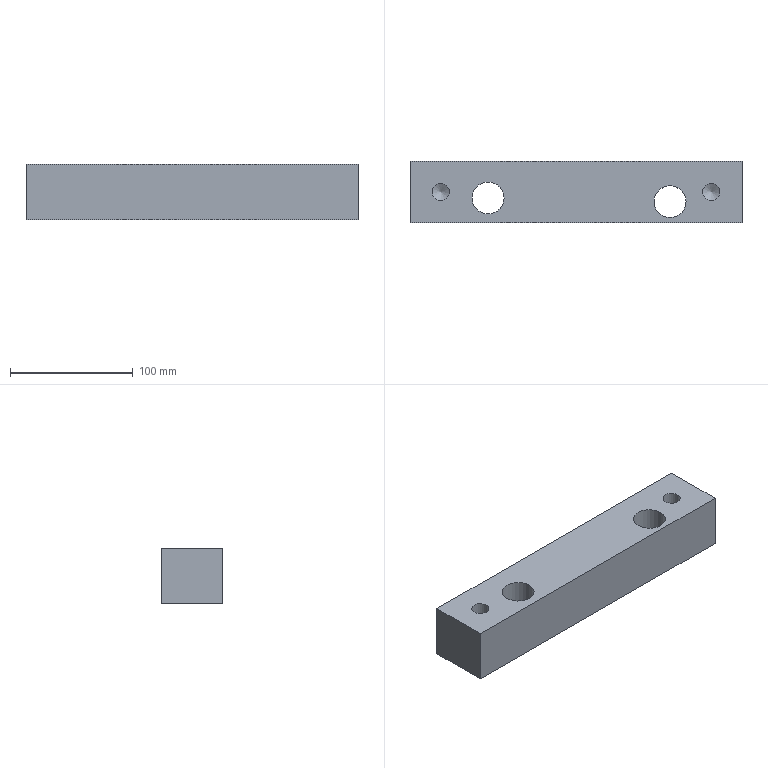Part | STEP file | 017_id2174_x_t | 1 solid | 12 faces | box 270 x 50 x 45 mm | volume 553311 mm3 | plane 6 | cylinder 4 | cone 2 | commonest cylinder face diameters 14 x2 26 x2
STEP:
#1=CARTESIAN_POINT('',(0.,0.,0.));
#2=DIRECTION('',(0.,0.,1.));
#3=DIRECTION('',(1.,0.,0.));
#4=AXIS2_PLACEMENT_3D('',#1,#2,#3);
#5=CARTESIAN_POINT('',(92.98,-48.947,230.));
#6=VERTEX_POINT('',#5);
#7=CARTESIAN_POINT('',(79.98,-48.947,230.));
#8=DIRECTION('',(0.,0.,1.));
#9=DIRECTION('',(1.,0.,0.));
#10=AXIS2_PLACEMENT_3D('',#7,#8,#9);
#11=CIRCLE('',#10,13.);
#12=CARTESIAN_POINT('',(303.5,139.,230.));
#13=DIRECTION('',(0.,0.,1.));
#14=DIRECTION('',(0.,1.,0.));
#15=AXIS2_PLACEMENT_3D('',#12,#13,#14);
#16=PLANE('',#15);
#17=CARTESIAN_POINT('',(-187.947,223.52));
#18=DIRECTION('',(0.,-1.));
#19=AXIS2_PLACEMENT_2D('',#17,#18);
#20=CIRCLE('',#19,13.);
#21=(GEOMETRIC_REPRESENTATION_CONTEXT(2)PARAMETRIC_REPRESENTATION_CONTEXT()REPRESENTATION_CONTEXT('',''));
#22=DEFINITIONAL_REPRESENTATION('',(#20),#21);
#23=PCURVE('',#16,#22);
#24=CARTESIAN_POINT('',(79.98,-48.947,360.));
#25=DIRECTION('',(0.,0.,-1.));
#26=DIRECTION('',(-1.,0.,0.));
#27=AXIS2_PLACEMENT_3D('',#24,#25,#26);
#28=CYLINDRICAL_SURFACE('',#27,13.);
#29=CARTESIAN_POINT('',(9.425,130.));
#30=DIRECTION('',(-1.,0.));
#31=VECTOR('',#30,1.);
#32=LINE('',#29,#31);
#33=(GEOMETRIC_REPRESENTATION_CONTEXT(2)PARAMETRIC_REPRESENTATION_CONTEXT()REPRESENTATION_CONTEXT('',''));
#34=DEFINITIONAL_REPRESENTATION('',(#32),#33);
#35=PCURVE('',#28,#34);
#36=SURFACE_CURVE('',#11,(#23,#35),.PCURVE_S1.);
#37=EDGE_CURVE('',#6,#6,#36,.T.);
#38=ORIENTED_EDGE('',*,*,#37,.F.);
#39=EDGE_LOOP('',(#38));
#40=FACE_BOUND('',#39,.T.);
#41=CARTESIAN_POINT('',(-55.02,-45.947,230.));
#42=VERTEX_POINT('',#41);
#43=CARTESIAN_POINT('',(-68.02,-45.947,230.));
#44=DIRECTION('',(0.,0.,1.));
#45=DIRECTION('',(1.,0.,0.));
#46=AXIS2_PLACEMENT_3D('',#43,#44,#45);
#47=CIRCLE('',#46,13.);
#48=CARTESIAN_POINT('',(-184.947,371.52));
#49=DIRECTION('',(0.,-1.));
#50=AXIS2_PLACEMENT_2D('',#48,#49);
#51=CIRCLE('',#50,13.);
#52=(GEOMETRIC_REPRESENTATION_CONTEXT(2)PARAMETRIC_REPRESENTATION_CONTEXT()REPRESENTATION_CONTEXT('',''));
#53=DEFINITIONAL_REPRESENTATION('',(#51),#52);
#54=PCURVE('',#16,#53);
#55=CARTESIAN_POINT('',(-68.02,-45.947,360.));
#56=DIRECTION('',(0.,0.,-1.));
#57=DIRECTION('',(-1.,0.,0.));
#58=AXIS2_PLACEMENT_3D('',#55,#56,#57);
#59=CYLINDRICAL_SURFACE('',#58,13.);
#60=CARTESIAN_POINT('',(9.425,130.));
#61=DIRECTION('',(-1.,0.));
#62=VECTOR('',#61,1.);
#63=LINE('',#60,#62);
#64=(GEOMETRIC_REPRESENTATION_CONTEXT(2)PARAMETRIC_REPRESENTATION_CONTEXT()REPRESENTATION_CONTEXT('',''));
#65=DEFINITIONAL_REPRESENTATION('',(#63),#64);
#66=PCURVE('',#59,#65);
#67=SURFACE_CURVE('',#47,(#54,#66),.PCURVE_S1.);
#68=EDGE_CURVE('',#42,#42,#67,.T.);
#69=ORIENTED_EDGE('',*,*,#68,.F.);
#70=EDGE_LOOP('',(#69));
#71=FACE_BOUND('',#70,.T.);
#72=CARTESIAN_POINT('',(-106.5,-48.,230.));
#73=VERTEX_POINT('',#72);
#74=CARTESIAN_POINT('',(-106.5,-34.,230.));
#75=VERTEX_POINT('',#74);
#76=CARTESIAN_POINT('',(-106.5,-41.,230.));
#77=DIRECTION('',(0.,0.,1.));
#78=DIRECTION('',(0.,-1.,0.));
#79=AXIS2_PLACEMENT_3D('',#76,#77,#78);
#80=CIRCLE('',#79,7.);
#81=CARTESIAN_POINT('',(-180.,410.));
#82=DIRECTION('',(-1.,0.));
#83=AXIS2_PLACEMENT_2D('',#81,#82);
#84=CIRCLE('',#83,7.);
#85=(GEOMETRIC_REPRESENTATION_CONTEXT(2)PARAMETRIC_REPRESENTATION_CONTEXT()REPRESENTATION_CONTEXT('',''));
#86=DEFINITIONAL_REPRESENTATION('',(#84),#85);
#87=PCURVE('',#16,#86);
#88=CARTESIAN_POINT('',(-106.5,-41.,279.));
#89=DIRECTION('',(0.,0.,-1.));
#90=DIRECTION('',(0.,1.,0.));
#91=AXIS2_PLACEMENT_3D('',#88,#89,#90);
#92=CYLINDRICAL_SURFACE('',#91,7.);
#93=CARTESIAN_POINT('',(3.142,49.));
#94=DIRECTION('',(-1.,0.));
#95=VECTOR('',#94,1.);
#96=LINE('',#93,#95);
#97=(GEOMETRIC_REPRESENTATION_CONTEXT(2)PARAMETRIC_REPRESENTATION_CONTEXT()REPRESENTATION_CONTEXT('',''));
#98=DEFINITIONAL_REPRESENTATION('',(#96),#97);
#99=PCURVE('',#92,#98);
#100=SURFACE_CURVE('',#80,(#87,#99),.PCURVE_S1.);
#101=EDGE_CURVE('',#73,#75,#100,.T.);
#102=ORIENTED_EDGE('',*,*,#101,.F.);
#103=CARTESIAN_POINT('',(-106.5,-41.,230.));
#104=DIRECTION('',(0.,0.,1.));
#105=DIRECTION('',(0.,-1.,0.));
#106=AXIS2_PLACEMENT_3D('',#103,#104,#105);
#107=CIRCLE('',#106,7.);
#108=CARTESIAN_POINT('',(-180.,410.));
#109=DIRECTION('',(-1.,0.));
#110=AXIS2_PLACEMENT_2D('',#108,#109);
#111=CIRCLE('',#110,7.);
#112=(GEOMETRIC_REPRESENTATION_CONTEXT(2)PARAMETRIC_REPRESENTATION_CONTEXT()REPRESENTATION_CONTEXT('',''));
#113=DEFINITIONAL_REPRESENTATION('',(#111),#112);
#114=PCURVE('',#16,#113);
#115=CARTESIAN_POINT('',(9.425,49.));
#116=DIRECTION('',(-1.,0.));
#117=VECTOR('',#116,1.);
#118=LINE('',#115,#117);
#119=(GEOMETRIC_REPRESENTATION_CONTEXT(2)PARAMETRIC_REPRESENTATION_CONTEXT()REPRESENTATION_CONTEXT('',''));
#120=DEFINITIONAL_REPRESENTATION('',(#118),#119);
#121=PCURVE('',#92,#120);
#122=SURFACE_CURVE('',#107,(#114,#121),.PCURVE_S1.);
#123=EDGE_CURVE('',#75,#73,#122,.T.);
#124=ORIENTED_EDGE('',*,*,#123,.F.);
#125=EDGE_LOOP('',(#102,#124));
#126=FACE_BOUND('',#125,.T.);
#127=CARTESIAN_POINT('',(113.5,-48.,230.));
#128=VERTEX_POINT('',#127);
#129=CARTESIAN_POINT('',(113.5,-34.,230.));
#130=VERTEX_POINT('',#129);
#131=CARTESIAN_POINT('',(113.5,-41.,230.));
#132=DIRECTION('',(0.,0.,-1.));
#133=DIRECTION('',(0.,-1.,0.));
#134=AXIS2_PLACEMENT_3D('',#131,#132,#133);
#135=CIRCLE('',#134,7.);
#136=CARTESIAN_POINT('',(-187.,190.));
#137=CARTESIAN_POINT('',(-187.,202.124));
#138=CARTESIAN_POINT('',(-176.5,196.062));
#139=CARTESIAN_POINT('',(-166.,190.));
#140=CARTESIAN_POINT('',(-176.5,183.938));
#141=CARTESIAN_POINT('',(-187.,177.876));
#142=CARTESIAN_POINT('',(-187.,190.));
#143=(BOUNDED_CURVE()B_SPLINE_CURVE(2,(#136,#137,#138,#139,#140,#141,#142),.UNSPECIFIED.,.T.,.F.)B_SPLINE_CURVE_WITH_KNOTS((1,2,2,2,2,1),(-2.094,0.,2.094,4.189,6.283,8.378),.UNSPECIFIED.)CURVE()GEOMETRIC_REPRESENTATION_ITEM()RATIONAL_B_SPLINE_CURVE((1.,0.5,1.,0.5,1.,0.5,1.))REPRESENTATION_ITEM(''));
#144=(GEOMETRIC_REPRESENTATION_CONTEXT(2)PARAMETRIC_REPRESENTATION_CONTEXT()REPRESENTATION_CONTEXT('',''));
#145=DEFINITIONAL_REPRESENTATION('',(#143),#144);
#146=PCURVE('',#16,#145);
#147=CARTESIAN_POINT('',(113.5,-41.,279.));
#148=DIRECTION('',(0.,0.,-1.));
#149=DIRECTION('',(0.,1.,0.));
#150=AXIS2_PLACEMENT_3D('',#147,#148,#149);
#151=CYLINDRICAL_SURFACE('',#150,7.);
#152=CARTESIAN_POINT('',(3.142,49.));
#153=DIRECTION('',(1.,0.));
#154=VECTOR('',#153,1.);
#155=LINE('',#152,#154);
#156=(GEOMETRIC_REPRESENTATION_CONTEXT(2)PARAMETRIC_REPRESENTATION_CONTEXT()REPRESENTATION_CONTEXT('',''));
#157=DEFINITIONAL_REPRESENTATION('',(#155),#156);
#158=PCURVE('',#151,#157);
#159=SURFACE_CURVE('',#135,(#146,#158),.PCURVE_S1.);
#160=EDGE_CURVE('',#128,#130,#159,.T.);
#161=ORIENTED_EDGE('',*,*,#160,.T.);
#162=CARTESIAN_POINT('',(113.5,-41.,230.));
#163=DIRECTION('',(0.,0.,-1.));
#164=DIRECTION('',(0.,-1.,0.));
#165=AXIS2_PLACEMENT_3D('',#162,#163,#164);
#166=CIRCLE('',#165,7.);
#167=CARTESIAN_POINT('',(-187.,190.));
#168=CARTESIAN_POINT('',(-187.,202.124));
#169=CARTESIAN_POINT('',(-176.5,196.062));
#170=CARTESIAN_POINT('',(-166.,190.));
#171=CARTESIAN_POINT('',(-176.5,183.938));
#172=CARTESIAN_POINT('',(-187.,177.876));
#173=CARTESIAN_POINT('',(-187.,190.));
#174=(BOUNDED_CURVE()B_SPLINE_CURVE(2,(#167,#168,#169,#170,#171,#172,#173),.UNSPECIFIED.,.T.,.F.)B_SPLINE_CURVE_WITH_KNOTS((1,2,2,2,2,1),(-2.094,0.,2.094,4.189,6.283,8.378),.UNSPECIFIED.)CURVE()GEOMETRIC_REPRESENTATION_ITEM()RATIONAL_B_SPLINE_CURVE((1.,0.5,1.,0.5,1.,0.5,1.))REPRESENTATION_ITEM(''));
#175=(GEOMETRIC_REPRESENTATION_CONTEXT(2)PARAMETRIC_REPRESENTATION_CONTEXT()REPRESENTATION_CONTEXT('',''));
#176=DEFINITIONAL_REPRESENTATION('',(#174),#175);
#177=PCURVE('',#16,#176);
#178=CARTESIAN_POINT('',(-3.142,49.));
#179=DIRECTION('',(1.,0.));
#180=VECTOR('',#179,1.);
#181=LINE('',#178,#180);
#182=(GEOMETRIC_REPRESENTATION_CONTEXT(2)PARAMETRIC_REPRESENTATION_CONTEXT()REPRESENTATION_CONTEXT('',''));
#183=DEFINITIONAL_REPRESENTATION('',(#181),#182);
#184=PCURVE('',#151,#183);
#185=SURFACE_CURVE('',#166,(#177,#184),.PCURVE_S1.);
#186=EDGE_CURVE('',#130,#128,#185,.T.);
#187=ORIENTED_EDGE('',*,*,#186,.T.);
#188=EDGE_LOOP('',(#161,#187));
#189=FACE_BOUND('',#188,.T.);
#190=CARTESIAN_POINT('',(-131.5,-16.,230.));
#191=VERTEX_POINT('',#190);
#192=CARTESIAN_POINT('',(-131.5,-66.,230.));
#193=VERTEX_POINT('',#192);
#194=CARTESIAN_POINT('',(-131.5,-66.,230.));
#195=DIRECTION('',(0.,-1.,0.));
#196=VECTOR('',#195,1.);
#197=LINE('',#194,#196);
#198=CARTESIAN_POINT('',(-205.,435.));
#199=DIRECTION('',(-1.,0.));
#200=VECTOR('',#199,1.);
#201=LINE('',#198,#200);
#202=(GEOMETRIC_REPRESENTATION_CONTEXT(2)PARAMETRIC_REPRESENTATION_CONTEXT()REPRESENTATION_CONTEXT('',''));
#203=DEFINITIONAL_REPRESENTATION('',(#201),#202);
#204=PCURVE('',#16,#203);
#205=CARTESIAN_POINT('',(-131.5,-66.,428.5));
#206=DIRECTION('',(-1.,0.,0.));
#207=DIRECTION('',(0.,0.,1.));
#208=AXIS2_PLACEMENT_3D('',#205,#206,#207);
#209=PLANE('',#208);
#210=CARTESIAN_POINT('',(-198.5,0.));
#211=DIRECTION('',(0.,-1.));
#212=VECTOR('',#211,1.);
#213=LINE('',#210,#212);
#214=(GEOMETRIC_REPRESENTATION_CONTEXT(2)PARAMETRIC_REPRESENTATION_CONTEXT()REPRESENTATION_CONTEXT('',''));
#215=DEFINITIONAL_REPRESENTATION('',(#213),#214);
#216=PCURVE('',#209,#215);
#217=SURFACE_CURVE('',#197,(#204,#216),.PCURVE_S1.);
#218=EDGE_CURVE('',#191,#193,#217,.T.);
#219=ORIENTED_EDGE('',*,*,#218,.T.);
#220=CARTESIAN_POINT('',(138.5,-66.,230.));
#221=VERTEX_POINT('',#220);
#222=CARTESIAN_POINT('',(513.5,-66.,230.));
#223=DIRECTION('',(1.,0.,0.));
#224=VECTOR('',#223,1.);
#225=LINE('',#222,#224);
#226=CARTESIAN_POINT('',(-205.,-210.));
#227=DIRECTION('',(0.,-1.));
#228=VECTOR('',#227,1.);
#229=LINE('',#226,#228);
#230=(GEOMETRIC_REPRESENTATION_CONTEXT(2)PARAMETRIC_REPRESENTATION_CONTEXT()REPRESENTATION_CONTEXT('',''));
#231=DEFINITIONAL_REPRESENTATION('',(#229),#230);
#232=PCURVE('',#16,#231);
#233=CARTESIAN_POINT('',(513.5,-66.,428.5));
#234=DIRECTION('',(0.,-1.,0.));
#235=DIRECTION('',(0.,0.,-1.));
#236=AXIS2_PLACEMENT_3D('',#233,#234,#235);
#237=PLANE('',#236);
#238=CARTESIAN_POINT('',(198.5,0.));
#239=DIRECTION('',(0.,1.));
#240=VECTOR('',#239,1.);
#241=LINE('',#238,#240);
#242=(GEOMETRIC_REPRESENTATION_CONTEXT(2)PARAMETRIC_REPRESENTATION_CONTEXT()REPRESENTATION_CONTEXT('',''));
#243=DEFINITIONAL_REPRESENTATION('',(#241),#242);
#244=PCURVE('',#237,#243);
#245=SURFACE_CURVE('',#225,(#232,#244),.PCURVE_S1.);
#246=EDGE_CURVE('',#193,#221,#245,.T.);
#247=ORIENTED_EDGE('',*,*,#246,.T.);
#248=CARTESIAN_POINT('',(138.5,-16.,230.));
#249=VERTEX_POINT('',#248);
#250=CARTESIAN_POINT('',(138.5,-66.,230.));
#251=DIRECTION('',(0.,-1.,0.));
#252=VECTOR('',#251,1.);
#253=LINE('',#250,#252);
#254=CARTESIAN_POINT('',(-205.,165.));
#255=DIRECTION('',(-1.,0.));
#256=VECTOR('',#255,1.);
#257=LINE('',#254,#256);
#258=(GEOMETRIC_REPRESENTATION_CONTEXT(2)PARAMETRIC_REPRESENTATION_CONTEXT()REPRESENTATION_CONTEXT('',''));
#259=DEFINITIONAL_REPRESENTATION('',(#257),#258);
#260=PCURVE('',#16,#259);
#261=CARTESIAN_POINT('',(138.5,-66.,428.5));
#262=DIRECTION('',(-1.,0.,0.));
#263=DIRECTION('',(0.,0.,1.));
#264=AXIS2_PLACEMENT_3D('',#261,#262,#263);
#265=PLANE('',#264);
#266=CARTESIAN_POINT('',(-198.5,0.));
#267=DIRECTION('',(0.,-1.));
#268=VECTOR('',#267,1.);
#269=LINE('',#266,#268);
#270=(GEOMETRIC_REPRESENTATION_CONTEXT(2)PARAMETRIC_REPRESENTATION_CONTEXT()REPRESENTATION_CONTEXT('',''));
#271=DEFINITIONAL_REPRESENTATION('',(#269),#270);
#272=PCURVE('',#265,#271);
#273=SURFACE_CURVE('',#253,(#260,#272),.PCURVE_S1.);
#274=EDGE_CURVE('',#249,#221,#273,.T.);
#275=ORIENTED_EDGE('',*,*,#274,.F.);
#276=CARTESIAN_POINT('',(513.5,-16.,230.));
#277=DIRECTION('',(-1.,0.,0.));
#278=VECTOR('',#277,1.);
#279=LINE('',#276,#278);
#280=CARTESIAN_POINT('',(-155.,-210.));
#281=DIRECTION('',(0.,1.));
#282=VECTOR('',#281,1.);
#283=LINE('',#280,#282);
#284=(GEOMETRIC_REPRESENTATION_CONTEXT(2)PARAMETRIC_REPRESENTATION_CONTEXT()REPRESENTATION_CONTEXT('',''));
#285=DEFINITIONAL_REPRESENTATION('',(#283),#284);
#286=PCURVE('',#16,#285);
#287=CARTESIAN_POINT('',(513.5,-16.,428.5));
#288=DIRECTION('',(0.,-1.,0.));
#289=DIRECTION('',(0.,0.,-1.));
#290=AXIS2_PLACEMENT_3D('',#287,#288,#289);
#291=PLANE('',#290);
#292=CARTESIAN_POINT('',(198.5,0.));
#293=DIRECTION('',(0.,-1.));
#294=VECTOR('',#293,1.);
#295=LINE('',#292,#294);
#296=(GEOMETRIC_REPRESENTATION_CONTEXT(2)PARAMETRIC_REPRESENTATION_CONTEXT()REPRESENTATION_CONTEXT('',''));
#297=DEFINITIONAL_REPRESENTATION('',(#295),#296);
#298=PCURVE('',#291,#297);
#299=SURFACE_CURVE('',#279,(#286,#298),.PCURVE_S1.);
#300=EDGE_CURVE('',#249,#191,#299,.T.);
#301=ORIENTED_EDGE('',*,*,#300,.T.);
#302=EDGE_LOOP('',(#219,#247,#275,#301));
#303=FACE_BOUND('',#302,.T.);
#304=ADVANCED_FACE('',(#40,#71,#126,#189,#303),#16,.T.);
#305=CARTESIAN_POINT('',(92.98,-48.947,185.));
#306=VERTEX_POINT('',#305);
#307=CARTESIAN_POINT('',(79.98,-48.947,185.));
#308=DIRECTION('',(0.,0.,1.));
#309=DIRECTION('',(1.,0.,0.));
#310=AXIS2_PLACEMENT_3D('',#307,#308,#309);
#311=CIRCLE('',#310,13.);
#312=CARTESIAN_POINT('',(513.5,-66.,185.));
#313=DIRECTION('',(0.,0.,1.));
#314=DIRECTION('',(1.,0.,0.));
#315=AXIS2_PLACEMENT_3D('',#312,#313,#314);
#316=PLANE('',#315);
#317=CARTESIAN_POINT('',(-433.52,17.053));
#318=DIRECTION('',(1.,0.));
#319=AXIS2_PLACEMENT_2D('',#317,#318);
#320=CIRCLE('',#319,13.);
#321=(GEOMETRIC_REPRESENTATION_CONTEXT(2)PARAMETRIC_REPRESENTATION_CONTEXT()REPRESENTATION_CONTEXT('',''));
#322=DEFINITIONAL_REPRESENTATION('',(#320),#321);
#323=PCURVE('',#316,#322);
#324=CARTESIAN_POINT('',(9.425,175.));
#325=DIRECTION('',(-1.,0.));
#326=VECTOR('',#325,1.);
#327=LINE('',#324,#326);
#328=(GEOMETRIC_REPRESENTATION_CONTEXT(2)PARAMETRIC_REPRESENTATION_CONTEXT()REPRESENTATION_CONTEXT('',''));
#329=DEFINITIONAL_REPRESENTATION('',(#327),#328);
#330=PCURVE('',#28,#329);
#331=SURFACE_CURVE('',#311,(#323,#330),.PCURVE_S1.);
#332=EDGE_CURVE('',#306,#306,#331,.T.);
#333=ORIENTED_EDGE('',*,*,#332,.T.);
#334=EDGE_LOOP('',(#333));
#335=FACE_BOUND('',#334,.T.);
#336=CARTESIAN_POINT('',(-55.02,-45.947,185.));
#337=VERTEX_POINT('',#336);
#338=CARTESIAN_POINT('',(-68.02,-45.947,185.));
#339=DIRECTION('',(0.,0.,1.));
#340=DIRECTION('',(1.,0.,0.));
#341=AXIS2_PLACEMENT_3D('',#338,#339,#340);
#342=CIRCLE('',#341,13.);
#343=CARTESIAN_POINT('',(-581.52,20.053));
#344=DIRECTION('',(1.,0.));
#345=AXIS2_PLACEMENT_2D('',#343,#344);
#346=CIRCLE('',#345,13.);
#347=(GEOMETRIC_REPRESENTATION_CONTEXT(2)PARAMETRIC_REPRESENTATION_CONTEXT()REPRESENTATION_CONTEXT('',''));
#348=DEFINITIONAL_REPRESENTATION('',(#346),#347);
#349=PCURVE('',#316,#348);
#350=CARTESIAN_POINT('',(9.425,175.));
#351=DIRECTION('',(-1.,0.));
#352=VECTOR('',#351,1.);
#353=LINE('',#350,#352);
#354=(GEOMETRIC_REPRESENTATION_CONTEXT(2)PARAMETRIC_REPRESENTATION_CONTEXT()REPRESENTATION_CONTEXT('',''));
#355=DEFINITIONAL_REPRESENTATION('',(#353),#354);
#356=PCURVE('',#59,#355);
#357=SURFACE_CURVE('',#342,(#349,#356),.PCURVE_S1.);
#358=EDGE_CURVE('',#337,#337,#357,.T.);
#359=ORIENTED_EDGE('',*,*,#358,.T.);
#360=EDGE_LOOP('',(#359));
#361=FACE_BOUND('',#360,.T.);
#362=CARTESIAN_POINT('',(138.5,-16.,185.));
#363=VERTEX_POINT('',#362);
#364=CARTESIAN_POINT('',(138.5,-66.,185.));
#365=VERTEX_POINT('',#364);
#366=CARTESIAN_POINT('',(138.5,-66.,185.));
#367=DIRECTION('',(0.,-1.,0.));
#368=VECTOR('',#367,1.);
#369=LINE('',#366,#368);
#370=CARTESIAN_POINT('',(-375.,0.));
#371=DIRECTION('',(0.,-1.));
#372=VECTOR('',#371,1.);
#373=LINE('',#370,#372);
#374=(GEOMETRIC_REPRESENTATION_CONTEXT(2)PARAMETRIC_REPRESENTATION_CONTEXT()REPRESENTATION_CONTEXT('',''));
#375=DEFINITIONAL_REPRESENTATION('',(#373),#374);
#376=PCURVE('',#316,#375);
#377=CARTESIAN_POINT('',(-243.5,0.));
#378=DIRECTION('',(0.,-1.));
#379=VECTOR('',#378,1.);
#380=LINE('',#377,#379);
#381=(GEOMETRIC_REPRESENTATION_CONTEXT(2)PARAMETRIC_REPRESENTATION_CONTEXT()REPRESENTATION_CONTEXT('',''));
#382=DEFINITIONAL_REPRESENTATION('',(#380),#381);
#383=PCURVE('',#265,#382);
#384=SURFACE_CURVE('',#369,(#376,#383),.PCURVE_S1.);
#385=EDGE_CURVE('',#363,#365,#384,.T.);
#386=ORIENTED_EDGE('',*,*,#385,.T.);
#387=CARTESIAN_POINT('',(-131.5,-66.,185.));
#388=VERTEX_POINT('',#387);
#389=CARTESIAN_POINT('',(513.5,-66.,185.));
#390=DIRECTION('',(-1.,0.,0.));
#391=VECTOR('',#390,1.);
#392=LINE('',#389,#391);
#393=CARTESIAN_POINT('',(0.,0.));
#394=DIRECTION('',(-1.,0.));
#395=VECTOR('',#394,1.);
#396=LINE('',#393,#395);
#397=(GEOMETRIC_REPRESENTATION_CONTEXT(2)PARAMETRIC_REPRESENTATION_CONTEXT()REPRESENTATION_CONTEXT('',''));
#398=DEFINITIONAL_REPRESENTATION('',(#396),#397);
#399=PCURVE('',#316,#398);
#400=CARTESIAN_POINT('',(243.5,0.));
#401=DIRECTION('',(0.,-1.));
#402=VECTOR('',#401,1.);
#403=LINE('',#400,#402);
#404=(GEOMETRIC_REPRESENTATION_CONTEXT(2)PARAMETRIC_REPRESENTATION_CONTEXT()REPRESENTATION_CONTEXT('',''));
#405=DEFINITIONAL_REPRESENTATION('',(#403),#404);
#406=PCURVE('',#237,#405);
#407=SURFACE_CURVE('',#392,(#399,#406),.PCURVE_S1.);
#408=EDGE_CURVE('',#365,#388,#407,.T.);
#409=ORIENTED_EDGE('',*,*,#408,.T.);
#410=CARTESIAN_POINT('',(-131.5,-16.,185.));
#411=VERTEX_POINT('',#410);
#412=CARTESIAN_POINT('',(-131.5,-66.,185.));
#413=DIRECTION('',(0.,-1.,0.));
#414=VECTOR('',#413,1.);
#415=LINE('',#412,#414);
#416=CARTESIAN_POINT('',(-645.,0.));
#417=DIRECTION('',(0.,-1.));
#418=VECTOR('',#417,1.);
#419=LINE('',#416,#418);
#420=(GEOMETRIC_REPRESENTATION_CONTEXT(2)PARAMETRIC_REPRESENTATION_CONTEXT()REPRESENTATION_CONTEXT('',''));
#421=DEFINITIONAL_REPRESENTATION('',(#419),#420);
#422=PCURVE('',#316,#421);
#423=CARTESIAN_POINT('',(-243.5,0.));
#424=DIRECTION('',(0.,-1.));
#425=VECTOR('',#424,1.);
#426=LINE('',#423,#425);
#427=(GEOMETRIC_REPRESENTATION_CONTEXT(2)PARAMETRIC_REPRESENTATION_CONTEXT()REPRESENTATION_CONTEXT('',''));
#428=DEFINITIONAL_REPRESENTATION('',(#426),#427);
#429=PCURVE('',#209,#428);
#430=SURFACE_CURVE('',#415,(#422,#429),.PCURVE_S1.);
#431=EDGE_CURVE('',#411,#388,#430,.T.);
#432=ORIENTED_EDGE('',*,*,#431,.F.);
#433=CARTESIAN_POINT('',(513.5,-16.,185.));
#434=DIRECTION('',(-1.,0.,0.));
#435=VECTOR('',#434,1.);
#436=LINE('',#433,#435);
#437=CARTESIAN_POINT('',(0.,50.));
#438=DIRECTION('',(-1.,0.));
#439=VECTOR('',#438,1.);
#440=LINE('',#437,#439);
#441=(GEOMETRIC_REPRESENTATION_CONTEXT(2)PARAMETRIC_REPRESENTATION_CONTEXT()REPRESENTATION_CONTEXT('',''));
#442=DEFINITIONAL_REPRESENTATION('',(#440),#441);
#443=PCURVE('',#316,#442);
#444=CARTESIAN_POINT('',(243.5,0.));
#445=DIRECTION('',(0.,-1.));
#446=VECTOR('',#445,1.);
#447=LINE('',#444,#446);
#448=(GEOMETRIC_REPRESENTATION_CONTEXT(2)PARAMETRIC_REPRESENTATION_CONTEXT()REPRESENTATION_CONTEXT('',''));
#449=DEFINITIONAL_REPRESENTATION('',(#447),#448);
#450=PCURVE('',#291,#449);
#451=SURFACE_CURVE('',#436,(#443,#450),.PCURVE_S1.);
#452=EDGE_CURVE('',#363,#411,#451,.T.);
#453=ORIENTED_EDGE('',*,*,#452,.F.);
#454=EDGE_LOOP('',(#386,#409,#432,#453));
#455=FACE_BOUND('',#454,.T.);
#456=ADVANCED_FACE('',(#335,#361,#455),#316,.F.);
#457=ORIENTED_EDGE('',*,*,#300,.F.);
#458=CARTESIAN_POINT('',(138.5,-16.,428.5));
#459=DIRECTION('',(0.,0.,-1.));
#460=VECTOR('',#459,1.);
#461=LINE('',#458,#460);
#462=CARTESIAN_POINT('',(0.,-375.));
#463=DIRECTION('',(1.,0.));
#464=VECTOR('',#463,1.);
#465=LINE('',#462,#464);
#466=(GEOMETRIC_REPRESENTATION_CONTEXT(2)PARAMETRIC_REPRESENTATION_CONTEXT()REPRESENTATION_CONTEXT('',''));
#467=DEFINITIONAL_REPRESENTATION('',(#465),#466);
#468=PCURVE('',#291,#467);
#469=CARTESIAN_POINT('',(0.,50.));
#470=DIRECTION('',(-1.,0.));
#471=VECTOR('',#470,1.);
#472=LINE('',#469,#471);
#473=(GEOMETRIC_REPRESENTATION_CONTEXT(2)PARAMETRIC_REPRESENTATION_CONTEXT()REPRESENTATION_CONTEXT('',''));
#474=DEFINITIONAL_REPRESENTATION('',(#472),#473);
#475=PCURVE('',#265,#474);
#476=SURFACE_CURVE('',#461,(#468,#475),.PCURVE_S1.);
#477=EDGE_CURVE('',#249,#363,#476,.T.);
#478=ORIENTED_EDGE('',*,*,#477,.T.);
#479=ORIENTED_EDGE('',*,*,#452,.T.);
#480=CARTESIAN_POINT('',(-131.5,-16.,428.5));
#481=DIRECTION('',(0.,0.,1.));
#482=VECTOR('',#481,1.);
#483=LINE('',#480,#482);
#484=CARTESIAN_POINT('',(0.,-645.));
#485=DIRECTION('',(-1.,0.));
#486=VECTOR('',#485,1.);
#487=LINE('',#484,#486);
#488=(GEOMETRIC_REPRESENTATION_CONTEXT(2)PARAMETRIC_REPRESENTATION_CONTEXT()REPRESENTATION_CONTEXT('',''));
#489=DEFINITIONAL_REPRESENTATION('',(#487),#488);
#490=PCURVE('',#291,#489);
#491=CARTESIAN_POINT('',(0.,50.));
#492=DIRECTION('',(1.,0.));
#493=VECTOR('',#492,1.);
#494=LINE('',#491,#493);
#495=(GEOMETRIC_REPRESENTATION_CONTEXT(2)PARAMETRIC_REPRESENTATION_CONTEXT()REPRESENTATION_CONTEXT('',''));
#496=DEFINITIONAL_REPRESENTATION('',(#494),#495);
#497=PCURVE('',#209,#496);
#498=SURFACE_CURVE('',#483,(#490,#497),.PCURVE_S1.);
#499=EDGE_CURVE('',#411,#191,#498,.T.);
#500=ORIENTED_EDGE('',*,*,#499,.T.);
#501=EDGE_LOOP('',(#457,#478,#479,#500));
#502=FACE_BOUND('',#501,.T.);
#503=ADVANCED_FACE('',(#502),#291,.F.);
#504=ORIENTED_EDGE('',*,*,#274,.T.);
#505=CARTESIAN_POINT('',(138.5,-66.,428.5));
#506=DIRECTION('',(0.,0.,-1.));
#507=VECTOR('',#506,1.);
#508=LINE('',#505,#507);
#509=CARTESIAN_POINT('',(0.,0.));
#510=DIRECTION('',(-1.,0.));
#511=VECTOR('',#510,1.);
#512=LINE('',#509,#511);
#513=(GEOMETRIC_REPRESENTATION_CONTEXT(2)PARAMETRIC_REPRESENTATION_CONTEXT()REPRESENTATION_CONTEXT('',''));
#514=DEFINITIONAL_REPRESENTATION('',(#512),#513);
#515=PCURVE('',#265,#514);
#516=CARTESIAN_POINT('',(0.,-375.));
#517=DIRECTION('',(1.,0.));
#518=VECTOR('',#517,1.);
#519=LINE('',#516,#518);
#520=(GEOMETRIC_REPRESENTATION_CONTEXT(2)PARAMETRIC_REPRESENTATION_CONTEXT()REPRESENTATION_CONTEXT('',''));
#521=DEFINITIONAL_REPRESENTATION('',(#519),#520);
#522=PCURVE('',#237,#521);
#523=SURFACE_CURVE('',#508,(#515,#522),.PCURVE_S1.);
#524=EDGE_CURVE('',#221,#365,#523,.T.);
#525=ORIENTED_EDGE('',*,*,#524,.T.);
#526=ORIENTED_EDGE('',*,*,#385,.F.);
#527=ORIENTED_EDGE('',*,*,#477,.F.);
#528=EDGE_LOOP('',(#504,#525,#526,#527));
#529=FACE_BOUND('',#528,.T.);
#530=ADVANCED_FACE('',(#529),#265,.F.);
#531=CARTESIAN_POINT('',(-131.5,-66.,428.5));
#532=DIRECTION('',(0.,0.,1.));
#533=VECTOR('',#532,1.);
#534=LINE('',#531,#533);
#535=CARTESIAN_POINT('',(0.,-645.));
#536=DIRECTION('',(-1.,0.));
#537=VECTOR('',#536,1.);
#538=LINE('',#535,#537);
#539=(GEOMETRIC_REPRESENTATION_CONTEXT(2)PARAMETRIC_REPRESENTATION_CONTEXT()REPRESENTATION_CONTEXT('',''));
#540=DEFINITIONAL_REPRESENTATION('',(#538),#539);
#541=PCURVE('',#237,#540);
#542=CARTESIAN_POINT('',(0.,0.));
#543=DIRECTION('',(1.,0.));
#544=VECTOR('',#543,1.);
#545=LINE('',#542,#544);
#546=(GEOMETRIC_REPRESENTATION_CONTEXT(2)PARAMETRIC_REPRESENTATION_CONTEXT()REPRESENTATION_CONTEXT('',''));
#547=DEFINITIONAL_REPRESENTATION('',(#545),#546);
#548=PCURVE('',#209,#547);
#549=SURFACE_CURVE('',#534,(#541,#548),.PCURVE_S1.);
#550=EDGE_CURVE('',#388,#193,#549,.T.);
#551=ORIENTED_EDGE('',*,*,#550,.F.);
#552=ORIENTED_EDGE('',*,*,#408,.F.);
#553=ORIENTED_EDGE('',*,*,#524,.F.);
#554=ORIENTED_EDGE('',*,*,#246,.F.);
#555=EDGE_LOOP('',(#551,#552,#553,#554));
#556=FACE_BOUND('',#555,.T.);
#557=ADVANCED_FACE('',(#556),#237,.T.);
#558=ORIENTED_EDGE('',*,*,#499,.F.);
#559=ORIENTED_EDGE('',*,*,#431,.T.);
#560=ORIENTED_EDGE('',*,*,#550,.T.);
#561=ORIENTED_EDGE('',*,*,#218,.F.);
#562=EDGE_LOOP('',(#558,#559,#560,#561));
#563=FACE_BOUND('',#562,.T.);
#564=ADVANCED_FACE('',(#563),#209,.T.);
#565=ORIENTED_EDGE('',*,*,#123,.F.);
#566=CARTESIAN_POINT('',(-106.5,-34.,210.541));
#567=VERTEX_POINT('',#566);
#568=CARTESIAN_POINT('',(-106.5,-34.,230.));
#569=CARTESIAN_POINT('',(-106.5,-34.,210.541));
#570=B_SPLINE_CURVE_WITH_KNOTS('',1,(#568,#569),.UNSPECIFIED.,.F.,.F.,(2,2),(49.,68.459),.PIECEWISE_BEZIER_KNOTS.);
#571=CARTESIAN_POINT('',(6.283,0.));
#572=DIRECTION('',(0.,1.));
#573=VECTOR('',#572,1.);
#574=LINE('',#571,#573);
#575=(GEOMETRIC_REPRESENTATION_CONTEXT(2)PARAMETRIC_REPRESENTATION_CONTEXT()REPRESENTATION_CONTEXT('',''));
#576=DEFINITIONAL_REPRESENTATION('',(#574),#575);
#577=PCURVE('',#92,#576);
#578=CARTESIAN_POINT('',(0.,0.));
#579=DIRECTION('',(0.,1.));
#580=VECTOR('',#579,1.);
#581=LINE('',#578,#580);
#582=(GEOMETRIC_REPRESENTATION_CONTEXT(2)PARAMETRIC_REPRESENTATION_CONTEXT()REPRESENTATION_CONTEXT('',''));
#583=DEFINITIONAL_REPRESENTATION('',(#581),#582);
#584=PCURVE('',#92,#583);
#585=SEAM_CURVE('',#570,(#577,#584),.PCURVE_S1.);
#586=EDGE_CURVE('',#75,#567,#585,.T.);
#587=ORIENTED_EDGE('',*,*,#586,.T.);
#588=CARTESIAN_POINT('',(-106.5,-48.,210.541));
#589=VERTEX_POINT('',#588);
#590=CARTESIAN_POINT('',(-106.5,-41.,210.541));
#591=DIRECTION('',(0.,0.,1.));
#592=DIRECTION('',(0.,1.,0.));
#593=AXIS2_PLACEMENT_3D('',#590,#591,#592);
#594=CIRCLE('',#593,7.);
#595=CARTESIAN_POINT('',(6.283,68.459));
#596=DIRECTION('',(-1.,0.));
#597=VECTOR('',#596,1.);
#598=LINE('',#595,#597);
#599=(GEOMETRIC_REPRESENTATION_CONTEXT(2)PARAMETRIC_REPRESENTATION_CONTEXT()REPRESENTATION_CONTEXT('',''));
#600=DEFINITIONAL_REPRESENTATION('',(#598),#599);
#601=PCURVE('',#92,#600);
#602=CARTESIAN_POINT('',(-106.5,-41.,210.541));
#603=DIRECTION('',(0.,0.,1.));
#604=DIRECTION('',(0.,-1.,0.));
#605=AXIS2_PLACEMENT_3D('',#602,#603,#604);
#606=CONICAL_SURFACE('',#605,7.,1.047);
#607=CARTESIAN_POINT('',(3.142,0.));
#608=DIRECTION('',(1.,0.));
#609=VECTOR('',#608,1.);
#610=LINE('',#607,#609);
#611=(GEOMETRIC_REPRESENTATION_CONTEXT(2)PARAMETRIC_REPRESENTATION_CONTEXT()REPRESENTATION_CONTEXT('',''));
#612=DEFINITIONAL_REPRESENTATION('',(#610),#611);
#613=PCURVE('',#606,#612);
#614=SURFACE_CURVE('',#594,(#601,#613),.PCURVE_S1.);
#615=EDGE_CURVE('',#567,#589,#614,.T.);
#616=ORIENTED_EDGE('',*,*,#615,.T.);
#617=CARTESIAN_POINT('',(-106.5,-41.,210.541));
#618=DIRECTION('',(0.,0.,1.));
#619=DIRECTION('',(0.,1.,0.));
#620=AXIS2_PLACEMENT_3D('',#617,#618,#619);
#621=CIRCLE('',#620,7.);
#622=CARTESIAN_POINT('',(6.283,68.459));
#623=DIRECTION('',(-1.,0.));
#624=VECTOR('',#623,1.);
#625=LINE('',#622,#624);
#626=(GEOMETRIC_REPRESENTATION_CONTEXT(2)PARAMETRIC_REPRESENTATION_CONTEXT()REPRESENTATION_CONTEXT('',''));
#627=DEFINITIONAL_REPRESENTATION('',(#625),#626);
#628=PCURVE('',#92,#627);
#629=CARTESIAN_POINT('',(-3.142,0.));
#630=DIRECTION('',(1.,0.));
#631=VECTOR('',#630,1.);
#632=LINE('',#629,#631);
#633=(GEOMETRIC_REPRESENTATION_CONTEXT(2)PARAMETRIC_REPRESENTATION_CONTEXT()REPRESENTATION_CONTEXT('',''));
#634=DEFINITIONAL_REPRESENTATION('',(#632),#633);
#635=PCURVE('',#606,#634);
#636=SURFACE_CURVE('',#621,(#628,#635),.PCURVE_S1.);
#637=EDGE_CURVE('',#589,#567,#636,.T.);
#638=ORIENTED_EDGE('',*,*,#637,.T.);
#639=ORIENTED_EDGE('',*,*,#586,.F.);
#640=ORIENTED_EDGE('',*,*,#101,.F.);
#641=EDGE_LOOP('',(#565,#587,#616,#638,#639,#640));
#642=FACE_BOUND('',#641,.F.);
#643=ADVANCED_FACE('',(#642),#92,.F.);
#644=CARTESIAN_POINT('',(-106.5,-41.,206.5));
#645=VERTEX_POINT('',#644);
#646=CARTESIAN_POINT('',(-106.5,-41.,206.5));
#647=CARTESIAN_POINT('',(-106.5,-48.,210.541));
#648=B_SPLINE_CURVE_WITH_KNOTS('',1,(#646,#647),.UNSPECIFIED.,.F.,.F.,(2,2),(-8.083,0.),.PIECEWISE_BEZIER_KNOTS.);
#649=CARTESIAN_POINT('',(6.283,0.));
#650=DIRECTION('',(0.,1.));
#651=VECTOR('',#650,1.);
#652=LINE('',#649,#651);
#653=(GEOMETRIC_REPRESENTATION_CONTEXT(2)PARAMETRIC_REPRESENTATION_CONTEXT()REPRESENTATION_CONTEXT('',''));
#654=DEFINITIONAL_REPRESENTATION('',(#652),#653);
#655=PCURVE('',#606,#654);
#656=CARTESIAN_POINT('',(0.,0.));
#657=DIRECTION('',(0.,1.));
#658=VECTOR('',#657,1.);
#659=LINE('',#656,#658);
#660=(GEOMETRIC_REPRESENTATION_CONTEXT(2)PARAMETRIC_REPRESENTATION_CONTEXT()REPRESENTATION_CONTEXT('',''));
#661=DEFINITIONAL_REPRESENTATION('',(#659),#660);
#662=PCURVE('',#606,#661);
#663=SEAM_CURVE('',#648,(#655,#662),.PCURVE_S1.);
#664=EDGE_CURVE('',#645,#589,#663,.T.);
#665=ORIENTED_EDGE('',*,*,#664,.T.);
#666=ORIENTED_EDGE('',*,*,#615,.F.);
#667=ORIENTED_EDGE('',*,*,#637,.F.);
#668=ORIENTED_EDGE('',*,*,#664,.F.);
#669=EDGE_LOOP('',(#665,#666,#667,#668));
#670=FACE_BOUND('',#669,.F.);
#671=ADVANCED_FACE('',(#670),#606,.F.);
#672=ORIENTED_EDGE('',*,*,#160,.T.);
#673=CARTESIAN_POINT('',(113.5,-34.,210.541));
#674=VERTEX_POINT('',#673);
#675=CARTESIAN_POINT('',(113.5,-34.,230.));
#676=CARTESIAN_POINT('',(113.5,-34.,210.541));
#677=B_SPLINE_CURVE_WITH_KNOTS('',1,(#675,#676),.UNSPECIFIED.,.F.,.F.,(2,2),(49.,68.459),.PIECEWISE_BEZIER_KNOTS.);
#678=CARTESIAN_POINT('',(6.283,0.));
#679=DIRECTION('',(0.,1.));
#680=VECTOR('',#679,1.);
#681=LINE('',#678,#680);
#682=(GEOMETRIC_REPRESENTATION_CONTEXT(2)PARAMETRIC_REPRESENTATION_CONTEXT()REPRESENTATION_CONTEXT('',''));
#683=DEFINITIONAL_REPRESENTATION('',(#681),#682);
#684=PCURVE('',#151,#683);
#685=CARTESIAN_POINT('',(0.,0.));
#686=DIRECTION('',(0.,1.));
#687=VECTOR('',#686,1.);
#688=LINE('',#685,#687);
#689=(GEOMETRIC_REPRESENTATION_CONTEXT(2)PARAMETRIC_REPRESENTATION_CONTEXT()REPRESENTATION_CONTEXT('',''));
#690=DEFINITIONAL_REPRESENTATION('',(#688),#689);
#691=PCURVE('',#151,#690);
#692=SEAM_CURVE('',#677,(#684,#691),.PCURVE_S1.);
#693=EDGE_CURVE('',#130,#674,#692,.T.);
#694=ORIENTED_EDGE('',*,*,#693,.T.);
#695=CARTESIAN_POINT('',(113.5,-48.,210.541));
#696=VERTEX_POINT('',#695);
#697=CARTESIAN_POINT('',(113.5,-41.,210.541));
#698=DIRECTION('',(0.,0.,-1.));
#699=DIRECTION('',(0.,1.,0.));
#700=AXIS2_PLACEMENT_3D('',#697,#698,#699);
#701=CIRCLE('',#700,7.);
#702=CARTESIAN_POINT('',(0.,68.459));
#703=DIRECTION('',(1.,0.));
#704=VECTOR('',#703,1.);
#705=LINE('',#702,#704);
#706=(GEOMETRIC_REPRESENTATION_CONTEXT(2)PARAMETRIC_REPRESENTATION_CONTEXT()REPRESENTATION_CONTEXT('',''));
#707=DEFINITIONAL_REPRESENTATION('',(#705),#706);
#708=PCURVE('',#151,#707);
#709=CARTESIAN_POINT('',(113.5,-41.,210.541));
#710=DIRECTION('',(0.,0.,1.));
#711=DIRECTION('',(0.,-1.,0.));
#712=AXIS2_PLACEMENT_3D('',#709,#710,#711);
#713=CONICAL_SURFACE('',#712,7.,1.047);
#714=CARTESIAN_POINT('',(9.425,0.));
#715=DIRECTION('',(-1.,0.));
#716=VECTOR('',#715,1.);
#717=LINE('',#714,#716);
#718=(GEOMETRIC_REPRESENTATION_CONTEXT(2)PARAMETRIC_REPRESENTATION_CONTEXT()REPRESENTATION_CONTEXT('',''));
#719=DEFINITIONAL_REPRESENTATION('',(#717),#718);
#720=PCURVE('',#713,#719);
#721=SURFACE_CURVE('',#701,(#708,#720),.PCURVE_S1.);
#722=EDGE_CURVE('',#696,#674,#721,.T.);
#723=ORIENTED_EDGE('',*,*,#722,.F.);
#724=CARTESIAN_POINT('',(113.5,-41.,210.541));
#725=DIRECTION('',(0.,0.,-1.));
#726=DIRECTION('',(0.,1.,0.));
#727=AXIS2_PLACEMENT_3D('',#724,#725,#726);
#728=CIRCLE('',#727,7.);
#729=CARTESIAN_POINT('',(0.,68.459));
#730=DIRECTION('',(1.,0.));
#731=VECTOR('',#730,1.);
#732=LINE('',#729,#731);
#733=(GEOMETRIC_REPRESENTATION_CONTEXT(2)PARAMETRIC_REPRESENTATION_CONTEXT()REPRESENTATION_CONTEXT('',''));
#734=DEFINITIONAL_REPRESENTATION('',(#732),#733);
#735=PCURVE('',#151,#734);
#736=CARTESIAN_POINT('',(3.142,0.));
#737=DIRECTION('',(-1.,0.));
#738=VECTOR('',#737,1.);
#739=LINE('',#736,#738);
#740=(GEOMETRIC_REPRESENTATION_CONTEXT(2)PARAMETRIC_REPRESENTATION_CONTEXT()REPRESENTATION_CONTEXT('',''));
#741=DEFINITIONAL_REPRESENTATION('',(#739),#740);
#742=PCURVE('',#713,#741);
#743=SURFACE_CURVE('',#728,(#735,#742),.PCURVE_S1.);
#744=EDGE_CURVE('',#674,#696,#743,.T.);
#745=ORIENTED_EDGE('',*,*,#744,.F.);
#746=ORIENTED_EDGE('',*,*,#693,.F.);
#747=ORIENTED_EDGE('',*,*,#186,.T.);
#748=EDGE_LOOP('',(#672,#694,#723,#745,#746,#747));
#749=FACE_BOUND('',#748,.F.);
#750=ADVANCED_FACE('',(#749),#151,.F.);
#751=CARTESIAN_POINT('',(113.5,-41.,206.5));
#752=VERTEX_POINT('',#751);
#753=CARTESIAN_POINT('',(113.5,-41.,206.5));
#754=CARTESIAN_POINT('',(113.5,-48.,210.541));
#755=B_SPLINE_CURVE_WITH_KNOTS('',1,(#753,#754),.UNSPECIFIED.,.F.,.F.,(2,2),(-8.083,0.),.PIECEWISE_BEZIER_KNOTS.);
#756=CARTESIAN_POINT('',(6.283,0.));
#757=DIRECTION('',(0.,1.));
#758=VECTOR('',#757,1.);
#759=LINE('',#756,#758);
#760=(GEOMETRIC_REPRESENTATION_CONTEXT(2)PARAMETRIC_REPRESENTATION_CONTEXT()REPRESENTATION_CONTEXT('',''));
#761=DEFINITIONAL_REPRESENTATION('',(#759),#760);
#762=PCURVE('',#713,#761);
#763=CARTESIAN_POINT('',(0.,0.));
#764=DIRECTION('',(0.,1.));
#765=VECTOR('',#764,1.);
#766=LINE('',#763,#765);
#767=(GEOMETRIC_REPRESENTATION_CONTEXT(2)PARAMETRIC_REPRESENTATION_CONTEXT()REPRESENTATION_CONTEXT('',''));
#768=DEFINITIONAL_REPRESENTATION('',(#766),#767);
#769=PCURVE('',#713,#768);
#770=SEAM_CURVE('',#755,(#762,#769),.PCURVE_S1.);
#771=EDGE_CURVE('',#752,#696,#770,.T.);
#772=ORIENTED_EDGE('',*,*,#771,.T.);
#773=ORIENTED_EDGE('',*,*,#722,.T.);
#774=ORIENTED_EDGE('',*,*,#744,.T.);
#775=ORIENTED_EDGE('',*,*,#771,.F.);
#776=EDGE_LOOP('',(#772,#773,#774,#775));
#777=FACE_BOUND('',#776,.F.);
#778=ADVANCED_FACE('',(#777),#713,.F.);
#779=ORIENTED_EDGE('',*,*,#68,.F.);
#780=CARTESIAN_POINT('',(-55.02,-45.947,230.));
#781=CARTESIAN_POINT('',(-55.02,-45.947,185.));
#782=B_SPLINE_CURVE_WITH_KNOTS('',1,(#780,#781),.UNSPECIFIED.,.F.,.F.,(2,2),(130.,175.),.PIECEWISE_BEZIER_KNOTS.);
#783=CARTESIAN_POINT('',(9.425,0.));
#784=DIRECTION('',(0.,1.));
#785=VECTOR('',#784,1.);
#786=LINE('',#783,#785);
#787=(GEOMETRIC_REPRESENTATION_CONTEXT(2)PARAMETRIC_REPRESENTATION_CONTEXT()REPRESENTATION_CONTEXT('',''));
#788=DEFINITIONAL_REPRESENTATION('',(#786),#787);
#789=PCURVE('',#59,#788);
#790=CARTESIAN_POINT('',(3.142,0.));
#791=DIRECTION('',(0.,1.));
#792=VECTOR('',#791,1.);
#793=LINE('',#790,#792);
#794=(GEOMETRIC_REPRESENTATION_CONTEXT(2)PARAMETRIC_REPRESENTATION_CONTEXT()REPRESENTATION_CONTEXT('',''));
#795=DEFINITIONAL_REPRESENTATION('',(#793),#794);
#796=PCURVE('',#59,#795);
#797=SEAM_CURVE('',#782,(#789,#796),.PCURVE_S1.);
#798=EDGE_CURVE('',#42,#337,#797,.T.);
#799=ORIENTED_EDGE('',*,*,#798,.T.);
#800=ORIENTED_EDGE('',*,*,#358,.T.);
#801=ORIENTED_EDGE('',*,*,#798,.F.);
#802=EDGE_LOOP('',(#779,#799,#800,#801));
#803=FACE_BOUND('',#802,.F.);
#804=ADVANCED_FACE('',(#803),#59,.F.);
#805=ORIENTED_EDGE('',*,*,#37,.F.);
#806=CARTESIAN_POINT('',(92.98,-48.947,230.));
#807=CARTESIAN_POINT('',(92.98,-48.947,185.));
#808=B_SPLINE_CURVE_WITH_KNOTS('',1,(#806,#807),.UNSPECIFIED.,.F.,.F.,(2,2),(130.,175.),.PIECEWISE_BEZIER_KNOTS.);
#809=CARTESIAN_POINT('',(9.425,0.));
#810=DIRECTION('',(0.,1.));
#811=VECTOR('',#810,1.);
#812=LINE('',#809,#811);
#813=(GEOMETRIC_REPRESENTATION_CONTEXT(2)PARAMETRIC_REPRESENTATION_CONTEXT()REPRESENTATION_CONTEXT('',''));
#814=DEFINITIONAL_REPRESENTATION('',(#812),#813);
#815=PCURVE('',#28,#814);
#816=CARTESIAN_POINT('',(3.142,0.));
#817=DIRECTION('',(0.,1.));
#818=VECTOR('',#817,1.);
#819=LINE('',#816,#818);
#820=(GEOMETRIC_REPRESENTATION_CONTEXT(2)PARAMETRIC_REPRESENTATION_CONTEXT()REPRESENTATION_CONTEXT('',''));
#821=DEFINITIONAL_REPRESENTATION('',(#819),#820);
#822=PCURVE('',#28,#821);
#823=SEAM_CURVE('',#808,(#815,#822),.PCURVE_S1.);
#824=EDGE_CURVE('',#6,#306,#823,.T.);
#825=ORIENTED_EDGE('',*,*,#824,.T.);
#826=ORIENTED_EDGE('',*,*,#332,.T.);
#827=ORIENTED_EDGE('',*,*,#824,.F.);
#828=EDGE_LOOP('',(#805,#825,#826,#827));
#829=FACE_BOUND('',#828,.F.);
#830=ADVANCED_FACE('',(#829),#28,.F.);
#831=CLOSED_SHELL('',(#304,#456,#503,#530,#557,#564,#643,#671,#750,#778,#804,#830));
#832=MANIFOLD_SOLID_BREP('',#831);
#833=(LENGTH_UNIT()NAMED_UNIT(*)SI_UNIT(.MILLI.,.METRE.));
#834=UNCERTAINTY_MEASURE_WITH_UNIT(LENGTH_MEASURE(0.000005),#833,'','');
#835=(NAMED_UNIT(*)PLANE_ANGLE_UNIT()SI_UNIT($,.RADIAN.));
#836=(NAMED_UNIT(*)SI_UNIT($,.STERADIAN.)SOLID_ANGLE_UNIT());
#837=(GEOMETRIC_REPRESENTATION_CONTEXT(3)GLOBAL_UNCERTAINTY_ASSIGNED_CONTEXT((#834))GLOBAL_UNIT_ASSIGNED_CONTEXT((#833,#835,#836))REPRESENTATION_CONTEXT('',''));
#838=ADVANCED_BREP_SHAPE_REPRESENTATION('',(#4,#832),#837);